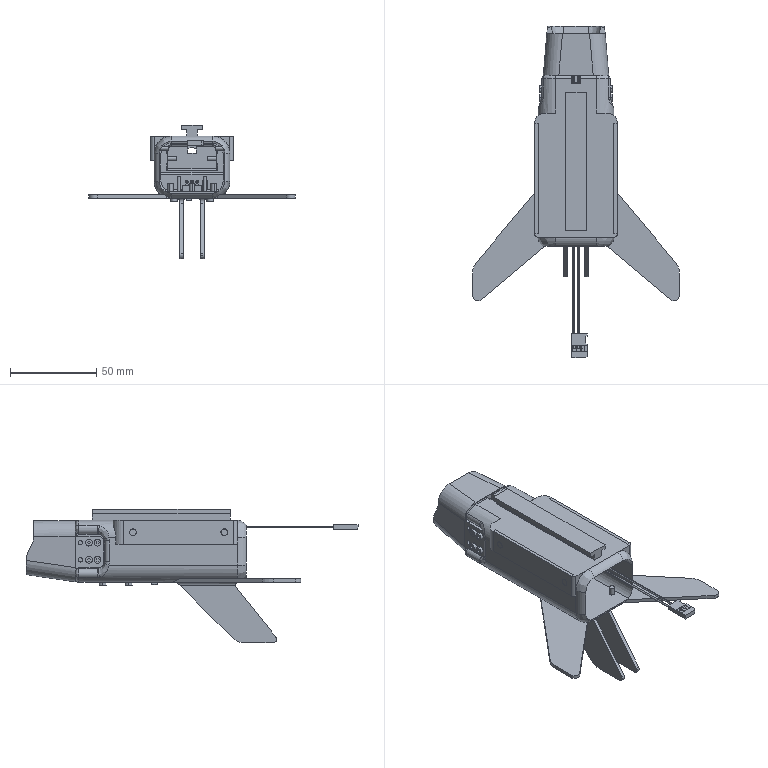Part | SolidWorks | 29 solids | 797 faces | box 120 x 192.5 x 77.3 mm | volume 102004 mm3 | plane 439 | cylinder 270 | spline 56 | cone 32 | commonest cylinder face diameters 2 x97 3.98 x28 2.5 x24 4 x16 0.2 x14 6 x14